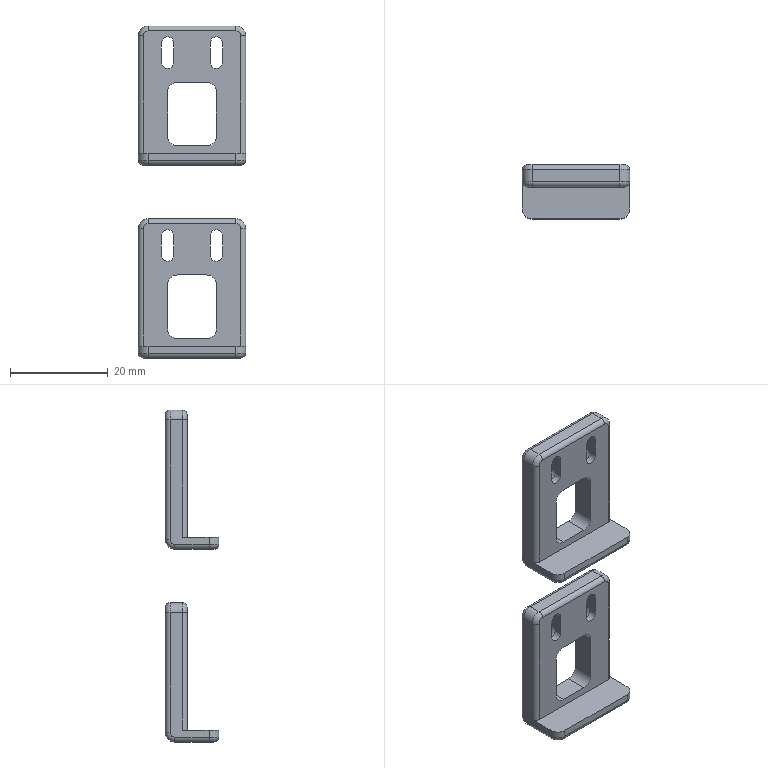Part | 2 solids | 112 faces | box 22 x 11 x 68 mm | volume 4626 mm3 | cylinder 52 | plane 44 | torus 16 | commonest cylinder face diameters 4 x26 2 x18 2.5 x8